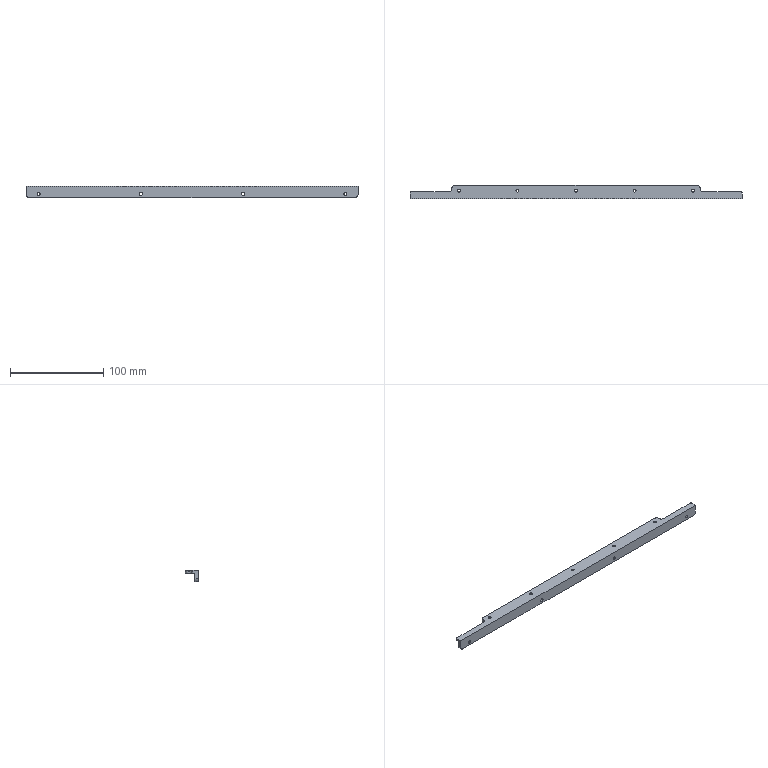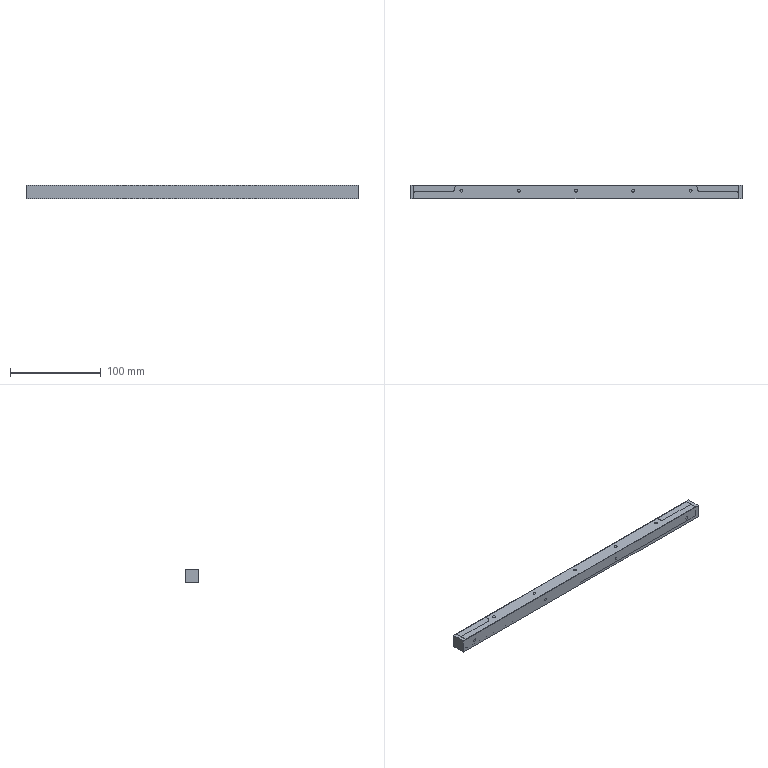CAM job | NX | 3+2 milling, drilling | part box 356.96 x 14 x 12 mm | stock box 365 x 15 x 15 mm
Tools:
number,name,description,diameter,corner_radius,flute_length,length,flutes
3,D6点钻,定心钻D6,6.0,0.0,57.0,93.0,2
1,D6开粗,D6,6.0,0.0,16.0,60.0,2
2,D6精光,D6,6.0,0.0,16.0,60.0,2
6,D16精光,D16,16.0,0.0,45.0,100.0,2
0,D4R0.5,圆鼻铣刀,4.0,0.5,12.0,50.0,2
0,Z3.3,Z3.3直柄钻头,3.3,0.0,36.0,65.0,2
2,M4X0.7,公制-铝用螺旋槽丝攻,3.3,0.0,13.0,21.0,2
4,D3.2,Drilling Tool,3.2,0.0,35.0,50.0,2
Operations:
program,operation,operation_type,tool,method,geometry_group,spindle_rpm,surface_speed,feed_per_tooth,feed_cut,feed_plunge,cut_length_mm,path_length_mm,cut_time_min,machine_time_min
XX-CNC1,PLANAR_MILL,PlanarMilling,D6开粗,METHOD,MCS_1,4500.0,100.0,0.1178,800.0,100.0,380.96,436.96,0.4762,0.4818
XX-CNC1,ADAPTIVE_MILLING,CavityMilling,D6开粗,METHOD,W1,6500.0,100.0,0.1178,3000.0,100.0,10359.27,19347.745,3.034,3.933
XX-CNC1,PLANAR_MILL_1,PlanarMilling,D6精光,METHOD,MCS_1,4500.0,100.0,0.1178,800.0,100.0,1524.897,1687.34,1.906,1.922
XX-CNC1,FLOOR_FACING,VolumeBased25DMillingOperation,D6精光,METHOD,MCS_1,4500.0,100.0,0.1178,800.0,100.0,1054.784,1126.784,1.319,1.326
XX-CNC1,PLANAR_MILL_1_COPY,PlanarMilling,D6精光,METHOD,MCS_1,4500.0,100.0,0.1178,800.0,100.0,371.36,445.36,0.4642,0.4716
XX-CNC1,DRILLING,Operation,D6点钻,METHOD,MCS_1,3000.0,0.0,0.0,200.0,0.0,27.5,397.286,0.1375,0.1745
XX-CNC1,PLANAR_MILL_2,PlanarMilling,D6点钻,METHOD,MCS_1,3500.0,100.0,0.1178,1000.0,100.0,723.92,848.92,0.7239,0.7364
XX-CNC1,PLANAR_MILL_2_COPY,PlanarMilling,D6点钻,METHOD,MCS_1,3500.0,100.0,0.1178,1000.0,100.0,375.81,453.81,0.3758,0.3836
XX-CNC1,DRILLING_COPY,Operation,D3.2,METHOD,MCS_1,3000.0,0.0,0.0,200.0,0.0,45.0,432.286,0.225,0.2637
XX-CNC1,CURVE_DRIVE,SurfaceContour,D4R0.5,METHOD,MCS_1,4500.0,56.0,0.1667,1500.0,100.0,970.613,1432.92,0.6471,0.6933
XX-CNC2,PLANAR_MILL_3,PlanarMilling,D16精光,METHOD,W2,4500.0,226.0,0.1333,1200.0,100.0,2321.76,4556.86,1.935,2.158
XX-CNC2,PLANAR_MILL_3_COPY,PlanarMilling,D16精光,METHOD,W2,4500.0,226.0,0.0889,800.0,100.0,386.96,442.96,0.4837,0.4893
XX-CNC2,PLANAR_MILL_4,PlanarMilling,D6点钻,METHOD,W2,3500.0,65.0,0.1429,1000.0,100.0,750.28,808.28,0.7503,0.7561
XX-CNC2,DRILLING_1,Operation,D6点钻,METHOD,W2,3000.0,56.0,0.05,300.0,0.0,23.0,370.286,0.0767,0.1114
XX-CNC3,DRILLING_2,Operation,D6点钻,METHOD,W3,2500.0,47.0,0.04,200.0,0.0,20.0,479.123,0.1,0.1459
XX-CNC3,DRILLING_2_COPY,Operation,Z3.3,METHOD,W3,2500.0,47.0,0.04,200.0,0.0,36.0,511.123,0.18,0.2275
XX-CNC3,DRILLING_2_COPY_1,Operation,M4X0.7,METHOD,W3,300.0,3.0,0.35,210.0,0.0,32.0,503.123,0.1524,0.1995